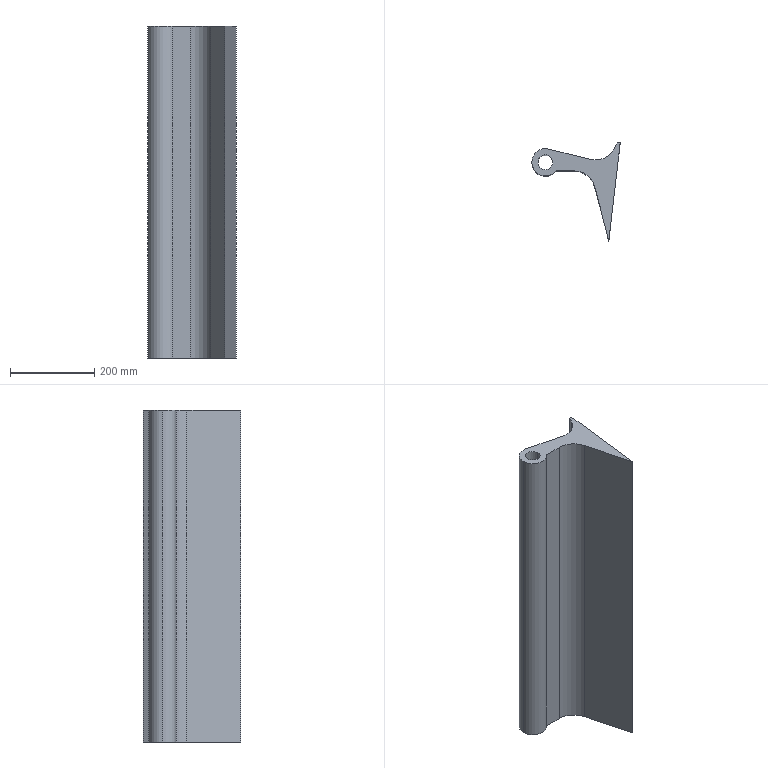Part | SolidWorks | features Fillet 2, Extrusion 1 | 1 solid | 14 faces | box 210.318 x 232.159 x 790 mm | volume 10438808 mm3 | plane 8 | cylinder 6 | commonest cylinder face diameters 35 x2 65 x2 100 x2
STEP:
#1=CARTESIAN_POINT('',(-17.5,0.,790.));
#2=VERTEX_POINT('',#1);
#3=CARTESIAN_POINT('',(17.5,0.,790.));
#4=VERTEX_POINT('',#3);
#5=CARTESIAN_POINT('',(0.,0.,790.));
#6=DIRECTION('',(0.,0.,1.));
#7=DIRECTION('',(1.,0.,0.));
#8=AXIS2_PLACEMENT_3D('',#5,#6,#7);
#9=CIRCLE('',#8,17.5);
#10=EDGE_CURVE('',#2,#4,#9,.T.);
#11=ORIENTED_EDGE('',*,*,#10,.T.);
#12=CARTESIAN_POINT('',(17.5,0.,0.));
#13=VERTEX_POINT('',#12);
#14=CARTESIAN_POINT('',(17.5,0.,790.));
#15=DIRECTION('',(0.,0.,-1.));
#16=VECTOR('',#15,1000.);
#17=LINE('',#14,#16);
#18=EDGE_CURVE('',#4,#13,#17,.T.);
#19=ORIENTED_EDGE('',*,*,#18,.T.);
#20=CARTESIAN_POINT('',(-17.5,0.,0.));
#21=VERTEX_POINT('',#20);
#22=CARTESIAN_POINT('',(0.,0.,0.));
#23=DIRECTION('',(0.,0.,1.));
#24=DIRECTION('',(1.,0.,0.));
#25=AXIS2_PLACEMENT_3D('',#22,#23,#24);
#26=CIRCLE('',#25,17.5);
#27=EDGE_CURVE('',#21,#13,#26,.T.);
#28=ORIENTED_EDGE('',*,*,#27,.F.);
#29=CARTESIAN_POINT('',(-17.5,0.,790.));
#30=DIRECTION('',(0.,0.,-1.));
#31=VECTOR('',#30,1000.);
#32=LINE('',#29,#31);
#33=EDGE_CURVE('',#2,#21,#32,.T.);
#34=ORIENTED_EDGE('',*,*,#33,.F.);
#35=EDGE_LOOP('',(#11,#19,#28,#34));
#36=FACE_OUTER_BOUND('',#35,.T.);
#37=CARTESIAN_POINT('',(0.,0.,790.));
#38=DIRECTION('',(0.,0.,-1.));
#39=DIRECTION('',(-1.,0.,0.));
#40=AXIS2_PLACEMENT_3D('',#37,#38,#39);
#41=CYLINDRICAL_SURFACE('',#40,17.5);
#42=ADVANCED_FACE('',(#36),#41,.F.);
#43=CARTESIAN_POINT('',(-32.5,0.,790.));
#44=VERTEX_POINT('',#43);
#45=CARTESIAN_POINT('',(25.188,-20.539,790.));
#46=VERTEX_POINT('',#45);
#47=CARTESIAN_POINT('',(0.,0.,790.));
#48=DIRECTION('',(0.,0.,1.));
#49=DIRECTION('',(1.,0.,0.));
#50=AXIS2_PLACEMENT_3D('',#47,#48,#49);
#51=CIRCLE('',#50,32.5);
#52=EDGE_CURVE('',#44,#46,#51,.T.);
#53=ORIENTED_EDGE('',*,*,#52,.F.);
#54=CARTESIAN_POINT('',(-32.5,0.,0.));
#55=VERTEX_POINT('',#54);
#56=CARTESIAN_POINT('',(-32.5,0.,790.));
#57=DIRECTION('',(0.,0.,-1.));
#58=VECTOR('',#57,1000.);
#59=LINE('',#56,#58);
#60=EDGE_CURVE('',#44,#55,#59,.T.);
#61=ORIENTED_EDGE('',*,*,#60,.T.);
#62=CARTESIAN_POINT('',(25.188,-20.539,0.));
#63=VERTEX_POINT('',#62);
#64=CARTESIAN_POINT('',(0.,0.,0.));
#65=DIRECTION('',(0.,0.,1.));
#66=DIRECTION('',(1.,0.,0.));
#67=AXIS2_PLACEMENT_3D('',#64,#65,#66);
#68=CIRCLE('',#67,32.5);
#69=EDGE_CURVE('',#55,#63,#68,.T.);
#70=ORIENTED_EDGE('',*,*,#69,.T.);
#71=CARTESIAN_POINT('',(25.188,-20.539,790.));
#72=DIRECTION('',(0.,0.,-1.));
#73=VECTOR('',#72,1000.);
#74=LINE('',#71,#73);
#75=EDGE_CURVE('',#46,#63,#74,.T.);
#76=ORIENTED_EDGE('',*,*,#75,.F.);
#77=EDGE_LOOP('',(#53,#61,#70,#76));
#78=FACE_OUTER_BOUND('',#77,.T.);
#79=CARTESIAN_POINT('',(0.,0.,790.));
#80=DIRECTION('',(0.,0.,-1.));
#81=DIRECTION('',(-1.,0.,0.));
#82=AXIS2_PLACEMENT_3D('',#79,#80,#81);
#83=CYLINDRICAL_SURFACE('',#82,32.5);
#84=ADVANCED_FACE('',(#78),#83,.T.);
#85=CARTESIAN_POINT('',(150.623,-186.13,790.));
#86=VERTEX_POINT('',#85);
#87=CARTESIAN_POINT('',(177.818,46.028,790.));
#88=VERTEX_POINT('',#87);
#89=CARTESIAN_POINT('',(150.623,-186.13,790.));
#90=DIRECTION('',(0.1163,0.9932,0.));
#91=VECTOR('',#90,1000.);
#92=LINE('',#89,#91);
#93=EDGE_CURVE('',#86,#88,#92,.T.);
#94=ORIENTED_EDGE('',*,*,#93,.T.);
#95=CARTESIAN_POINT('',(170.412,46.028,790.));
#96=VERTEX_POINT('',#95);
#97=CARTESIAN_POINT('',(177.818,46.028,790.));
#98=DIRECTION('',(-1.,0.,0.));
#99=VECTOR('',#98,1000.);
#100=LINE('',#97,#99);
#101=EDGE_CURVE('',#88,#96,#100,.T.);
#102=ORIENTED_EDGE('',*,*,#101,.T.);
#103=CARTESIAN_POINT('',(163.403,32.535,790.));
#104=VERTEX_POINT('',#103);
#105=CARTESIAN_POINT('',(145.258,-2.393,790.));
#106=DIRECTION('',(-0.461,-0.8874,0.));
#107=VECTOR('',#106,1000.);
#108=LINE('',#105,#107);
#109=EDGE_CURVE('',#96,#104,#108,.T.);
#110=ORIENTED_EDGE('',*,*,#109,.T.);
#111=CARTESIAN_POINT('',(107.046,7.043,790.));
#112=VERTEX_POINT('',#111);
#113=CARTESIAN_POINT('',(119.033,55.585,790.));
#114=DIRECTION('',(0.,0.,-1.));
#115=DIRECTION('',(1.,0.,0.));
#116=AXIS2_PLACEMENT_3D('',#113,#114,#115);
#117=CIRCLE('',#116,50.);
#118=EDGE_CURVE('',#104,#112,#117,.T.);
#119=ORIENTED_EDGE('',*,*,#118,.T.);
#120=CARTESIAN_POINT('',(7.791,31.552,790.));
#121=VERTEX_POINT('',#120);
#122=CARTESIAN_POINT('',(7.791,31.552,790.));
#123=DIRECTION('',(-0.9708,0.2397,0.));
#124=VECTOR('',#123,1000.);
#125=LINE('',#122,#124);
#126=EDGE_CURVE('',#112,#121,#125,.T.);
#127=ORIENTED_EDGE('',*,*,#126,.T.);
#128=CARTESIAN_POINT('',(0.,0.,790.));
#129=DIRECTION('',(0.,0.,1.));
#130=DIRECTION('',(1.,0.,0.));
#131=AXIS2_PLACEMENT_3D('',#128,#129,#130);
#132=CIRCLE('',#131,32.5);
#133=EDGE_CURVE('',#121,#44,#132,.T.);
#134=ORIENTED_EDGE('',*,*,#133,.T.);
#135=ORIENTED_EDGE('',*,*,#52,.T.);
#136=CARTESIAN_POINT('',(68.802,-20.539,790.));
#137=VERTEX_POINT('',#136);
#138=CARTESIAN_POINT('',(107.434,-20.539,790.));
#139=DIRECTION('',(1.,0.,0.));
#140=VECTOR('',#139,1000.);
#141=LINE('',#138,#140);
#142=EDGE_CURVE('',#46,#137,#141,.T.);
#143=ORIENTED_EDGE('',*,*,#142,.T.);
#144=CARTESIAN_POINT('',(117.184,-57.92,790.));
#145=VERTEX_POINT('',#144);
#146=CARTESIAN_POINT('',(68.802,-70.539,790.));
#147=DIRECTION('',(0.,0.,-1.));
#148=DIRECTION('',(1.,0.,0.));
#149=AXIS2_PLACEMENT_3D('',#146,#147,#148);
#150=CIRCLE('',#149,50.);
#151=EDGE_CURVE('',#137,#145,#150,.T.);
#152=ORIENTED_EDGE('',*,*,#151,.T.);
#153=CARTESIAN_POINT('',(107.434,-20.539,790.));
#154=DIRECTION('',(0.2524,-0.9676,0.));
#155=VECTOR('',#154,1000.);
#156=LINE('',#153,#155);
#157=EDGE_CURVE('',#145,#86,#156,.T.);
#158=ORIENTED_EDGE('',*,*,#157,.T.);
#159=EDGE_LOOP('',(#94,#102,#110,#119,#127,#134,#135,#143,#152,#158));
#160=FACE_OUTER_BOUND('',#159,.T.);
#161=ORIENTED_EDGE('',*,*,#10,.F.);
#162=CARTESIAN_POINT('',(0.,0.,790.));
#163=DIRECTION('',(0.,0.,1.));
#164=DIRECTION('',(1.,0.,0.));
#165=AXIS2_PLACEMENT_3D('',#162,#163,#164);
#166=CIRCLE('',#165,17.5);
#167=EDGE_CURVE('',#4,#2,#166,.T.);
#168=ORIENTED_EDGE('',*,*,#167,.F.);
#169=EDGE_LOOP('',(#161,#168));
#170=FACE_BOUND('',#169,.T.);
#171=CARTESIAN_POINT('',(0.,0.,790.));
#172=DIRECTION('',(0.,0.,1.));
#173=DIRECTION('',(1.,0.,0.));
#174=AXIS2_PLACEMENT_3D('',#171,#172,#173);
#175=PLANE('',#174);
#176=ADVANCED_FACE('',(#160,#170),#175,.T.);
#177=CARTESIAN_POINT('',(150.623,-186.13,0.));
#178=VERTEX_POINT('',#177);
#179=CARTESIAN_POINT('',(177.818,46.028,0.));
#180=VERTEX_POINT('',#179);
#181=CARTESIAN_POINT('',(150.623,-186.13,0.));
#182=DIRECTION('',(0.1163,0.9932,0.));
#183=VECTOR('',#182,1000.);
#184=LINE('',#181,#183);
#185=EDGE_CURVE('',#178,#180,#184,.T.);
#186=ORIENTED_EDGE('',*,*,#185,.F.);
#187=CARTESIAN_POINT('',(117.184,-57.92,0.));
#188=VERTEX_POINT('',#187);
#189=CARTESIAN_POINT('',(107.434,-20.539,0.));
#190=DIRECTION('',(0.2524,-0.9676,0.));
#191=VECTOR('',#190,1000.);
#192=LINE('',#189,#191);
#193=EDGE_CURVE('',#188,#178,#192,.T.);
#194=ORIENTED_EDGE('',*,*,#193,.F.);
#195=CARTESIAN_POINT('',(68.802,-20.539,0.));
#196=VERTEX_POINT('',#195);
#197=CARTESIAN_POINT('',(68.802,-70.539,0.));
#198=DIRECTION('',(0.,0.,1.));
#199=DIRECTION('',(1.,0.,0.));
#200=AXIS2_PLACEMENT_3D('',#197,#198,#199);
#201=CIRCLE('',#200,50.);
#202=EDGE_CURVE('',#188,#196,#201,.T.);
#203=ORIENTED_EDGE('',*,*,#202,.T.);
#204=CARTESIAN_POINT('',(107.434,-20.539,0.));
#205=DIRECTION('',(1.,0.,0.));
#206=VECTOR('',#205,1000.);
#207=LINE('',#204,#206);
#208=EDGE_CURVE('',#63,#196,#207,.T.);
#209=ORIENTED_EDGE('',*,*,#208,.F.);
#210=ORIENTED_EDGE('',*,*,#69,.F.);
#211=CARTESIAN_POINT('',(7.791,31.552,0.));
#212=VERTEX_POINT('',#211);
#213=CARTESIAN_POINT('',(0.,0.,0.));
#214=DIRECTION('',(0.,0.,1.));
#215=DIRECTION('',(1.,0.,0.));
#216=AXIS2_PLACEMENT_3D('',#213,#214,#215);
#217=CIRCLE('',#216,32.5);
#218=EDGE_CURVE('',#212,#55,#217,.T.);
#219=ORIENTED_EDGE('',*,*,#218,.F.);
#220=CARTESIAN_POINT('',(107.046,7.043,0.));
#221=VERTEX_POINT('',#220);
#222=CARTESIAN_POINT('',(7.791,31.552,0.));
#223=DIRECTION('',(-0.9708,0.2397,0.));
#224=VECTOR('',#223,1000.);
#225=LINE('',#222,#224);
#226=EDGE_CURVE('',#221,#212,#225,.T.);
#227=ORIENTED_EDGE('',*,*,#226,.F.);
#228=CARTESIAN_POINT('',(163.403,32.535,0.));
#229=VERTEX_POINT('',#228);
#230=CARTESIAN_POINT('',(119.033,55.585,0.));
#231=DIRECTION('',(0.,0.,1.));
#232=DIRECTION('',(1.,0.,0.));
#233=AXIS2_PLACEMENT_3D('',#230,#231,#232);
#234=CIRCLE('',#233,50.);
#235=EDGE_CURVE('',#221,#229,#234,.T.);
#236=ORIENTED_EDGE('',*,*,#235,.T.);
#237=CARTESIAN_POINT('',(170.412,46.028,0.));
#238=VERTEX_POINT('',#237);
#239=CARTESIAN_POINT('',(145.258,-2.393,0.));
#240=DIRECTION('',(-0.461,-0.8874,0.));
#241=VECTOR('',#240,1000.);
#242=LINE('',#239,#241);
#243=EDGE_CURVE('',#238,#229,#242,.T.);
#244=ORIENTED_EDGE('',*,*,#243,.F.);
#245=CARTESIAN_POINT('',(177.818,46.028,0.));
#246=DIRECTION('',(-1.,0.,0.));
#247=VECTOR('',#246,1000.);
#248=LINE('',#245,#247);
#249=EDGE_CURVE('',#180,#238,#248,.T.);
#250=ORIENTED_EDGE('',*,*,#249,.F.);
#251=EDGE_LOOP('',(#186,#194,#203,#209,#210,#219,#227,#236,#244,#250));
#252=FACE_OUTER_BOUND('',#251,.T.);
#253=ORIENTED_EDGE('',*,*,#27,.T.);
#254=CARTESIAN_POINT('',(0.,0.,0.));
#255=DIRECTION('',(0.,0.,1.));
#256=DIRECTION('',(1.,0.,0.));
#257=AXIS2_PLACEMENT_3D('',#254,#255,#256);
#258=CIRCLE('',#257,17.5);
#259=EDGE_CURVE('',#13,#21,#258,.T.);
#260=ORIENTED_EDGE('',*,*,#259,.T.);
#261=EDGE_LOOP('',(#253,#260));
#262=FACE_BOUND('',#261,.T.);
#263=CARTESIAN_POINT('',(0.,0.,0.));
#264=DIRECTION('',(0.,0.,1.));
#265=DIRECTION('',(1.,0.,0.));
#266=AXIS2_PLACEMENT_3D('',#263,#264,#265);
#267=PLANE('',#266);
#268=ADVANCED_FACE('',(#252,#262),#267,.F.);
#269=ORIENTED_EDGE('',*,*,#185,.T.);
#270=CARTESIAN_POINT('',(177.818,46.028,790.));
#271=DIRECTION('',(0.,0.,-1.));
#272=VECTOR('',#271,1000.);
#273=LINE('',#270,#272);
#274=EDGE_CURVE('',#88,#180,#273,.T.);
#275=ORIENTED_EDGE('',*,*,#274,.F.);
#276=ORIENTED_EDGE('',*,*,#93,.F.);
#277=CARTESIAN_POINT('',(150.623,-186.13,790.));
#278=DIRECTION('',(0.,0.,-1.));
#279=VECTOR('',#278,1000.);
#280=LINE('',#277,#279);
#281=EDGE_CURVE('',#86,#178,#280,.T.);
#282=ORIENTED_EDGE('',*,*,#281,.T.);
#283=EDGE_LOOP('',(#269,#275,#276,#282));
#284=FACE_OUTER_BOUND('',#283,.T.);
#285=CARTESIAN_POINT('',(150.623,-186.13,790.));
#286=DIRECTION('',(-0.9932,0.1163,0.));
#287=DIRECTION('',(-0.1163,-0.9932,0.));
#288=AXIS2_PLACEMENT_3D('',#285,#286,#287);
#289=PLANE('',#288);
#290=ADVANCED_FACE('',(#284),#289,.F.);
#291=ORIENTED_EDGE('',*,*,#249,.T.);
#292=CARTESIAN_POINT('',(170.412,46.028,790.));
#293=DIRECTION('',(0.,0.,-1.));
#294=VECTOR('',#293,1000.);
#295=LINE('',#292,#294);
#296=EDGE_CURVE('',#96,#238,#295,.T.);
#297=ORIENTED_EDGE('',*,*,#296,.F.);
#298=ORIENTED_EDGE('',*,*,#101,.F.);
#299=ORIENTED_EDGE('',*,*,#274,.T.);
#300=EDGE_LOOP('',(#291,#297,#298,#299));
#301=FACE_OUTER_BOUND('',#300,.T.);
#302=CARTESIAN_POINT('',(177.818,46.028,790.));
#303=DIRECTION('',(0.,-1.,0.));
#304=DIRECTION('',(0.,0.,-1.));
#305=AXIS2_PLACEMENT_3D('',#302,#303,#304);
#306=PLANE('',#305);
#307=ADVANCED_FACE('',(#301),#306,.F.);
#308=ORIENTED_EDGE('',*,*,#243,.T.);
#309=CARTESIAN_POINT('',(163.403,32.535,790.));
#310=DIRECTION('',(0.,0.,1.));
#311=VECTOR('',#310,1000.);
#312=LINE('',#309,#311);
#313=EDGE_CURVE('',#229,#104,#312,.T.);
#314=ORIENTED_EDGE('',*,*,#313,.T.);
#315=ORIENTED_EDGE('',*,*,#109,.F.);
#316=ORIENTED_EDGE('',*,*,#296,.T.);
#317=EDGE_LOOP('',(#308,#314,#315,#316));
#318=FACE_OUTER_BOUND('',#317,.T.);
#319=CARTESIAN_POINT('',(145.258,-2.393,790.));
#320=DIRECTION('',(0.8874,-0.461,0.));
#321=DIRECTION('',(0.461,0.8874,0.));
#322=AXIS2_PLACEMENT_3D('',#319,#320,#321);
#323=PLANE('',#322);
#324=ADVANCED_FACE('',(#318),#323,.F.);
#325=ORIENTED_EDGE('',*,*,#126,.F.);
#326=CARTESIAN_POINT('',(107.046,7.043,0.));
#327=DIRECTION('',(0.,0.,-1.));
#328=VECTOR('',#327,1000.);
#329=LINE('',#326,#328);
#330=EDGE_CURVE('',#112,#221,#329,.T.);
#331=ORIENTED_EDGE('',*,*,#330,.T.);
#332=ORIENTED_EDGE('',*,*,#226,.T.);
#333=CARTESIAN_POINT('',(7.791,31.552,790.));
#334=DIRECTION('',(0.,0.,-1.));
#335=VECTOR('',#334,1000.);
#336=LINE('',#333,#335);
#337=EDGE_CURVE('',#121,#212,#336,.T.);
#338=ORIENTED_EDGE('',*,*,#337,.F.);
#339=EDGE_LOOP('',(#325,#331,#332,#338));
#340=FACE_OUTER_BOUND('',#339,.T.);
#341=CARTESIAN_POINT('',(7.791,31.552,790.));
#342=DIRECTION('',(-0.2397,-0.9708,0.));
#343=DIRECTION('',(0.9708,-0.2397,0.));
#344=AXIS2_PLACEMENT_3D('',#341,#342,#343);
#345=PLANE('',#344);
#346=ADVANCED_FACE('',(#340),#345,.F.);
#347=ORIENTED_EDGE('',*,*,#60,.F.);
#348=ORIENTED_EDGE('',*,*,#133,.F.);
#349=ORIENTED_EDGE('',*,*,#337,.T.);
#350=ORIENTED_EDGE('',*,*,#218,.T.);
#351=EDGE_LOOP('',(#347,#348,#349,#350));
#352=FACE_OUTER_BOUND('',#351,.T.);
#353=CARTESIAN_POINT('',(0.,0.,790.));
#354=DIRECTION('',(0.,0.,-1.));
#355=DIRECTION('',(-1.,0.,0.));
#356=AXIS2_PLACEMENT_3D('',#353,#354,#355);
#357=CYLINDRICAL_SURFACE('',#356,32.5);
#358=ADVANCED_FACE('',(#352),#357,.T.);
#359=ORIENTED_EDGE('',*,*,#208,.T.);
#360=CARTESIAN_POINT('',(68.802,-20.539,790.));
#361=DIRECTION('',(0.,0.,1.));
#362=VECTOR('',#361,1000.);
#363=LINE('',#360,#362);
#364=EDGE_CURVE('',#196,#137,#363,.T.);
#365=ORIENTED_EDGE('',*,*,#364,.T.);
#366=ORIENTED_EDGE('',*,*,#142,.F.);
#367=ORIENTED_EDGE('',*,*,#75,.T.);
#368=EDGE_LOOP('',(#359,#365,#366,#367));
#369=FACE_OUTER_BOUND('',#368,.T.);
#370=CARTESIAN_POINT('',(107.434,-20.539,790.));
#371=DIRECTION('',(0.,1.,0.));
#372=DIRECTION('',(-1.,0.,0.));
#373=AXIS2_PLACEMENT_3D('',#370,#371,#372);
#374=PLANE('',#373);
#375=ADVANCED_FACE('',(#369),#374,.F.);
#376=ORIENTED_EDGE('',*,*,#157,.F.);
#377=CARTESIAN_POINT('',(117.184,-57.92,0.));
#378=DIRECTION('',(0.,0.,-1.));
#379=VECTOR('',#378,1000.);
#380=LINE('',#377,#379);
#381=EDGE_CURVE('',#145,#188,#380,.T.);
#382=ORIENTED_EDGE('',*,*,#381,.T.);
#383=ORIENTED_EDGE('',*,*,#193,.T.);
#384=ORIENTED_EDGE('',*,*,#281,.F.);
#385=EDGE_LOOP('',(#376,#382,#383,#384));
#386=FACE_OUTER_BOUND('',#385,.T.);
#387=CARTESIAN_POINT('',(107.434,-20.539,790.));
#388=DIRECTION('',(0.9676,0.2524,0.));
#389=DIRECTION('',(-0.2524,0.9676,0.));
#390=AXIS2_PLACEMENT_3D('',#387,#388,#389);
#391=PLANE('',#390);
#392=ADVANCED_FACE('',(#386),#391,.F.);
#393=ORIENTED_EDGE('',*,*,#18,.F.);
#394=ORIENTED_EDGE('',*,*,#167,.T.);
#395=ORIENTED_EDGE('',*,*,#33,.T.);
#396=ORIENTED_EDGE('',*,*,#259,.F.);
#397=EDGE_LOOP('',(#393,#394,#395,#396));
#398=FACE_OUTER_BOUND('',#397,.T.);
#399=CARTESIAN_POINT('',(0.,0.,790.));
#400=DIRECTION('',(0.,0.,-1.));
#401=DIRECTION('',(-1.,0.,0.));
#402=AXIS2_PLACEMENT_3D('',#399,#400,#401);
#403=CYLINDRICAL_SURFACE('',#402,17.5);
#404=ADVANCED_FACE('',(#398),#403,.F.);
#405=ORIENTED_EDGE('',*,*,#118,.F.);
#406=ORIENTED_EDGE('',*,*,#313,.F.);
#407=ORIENTED_EDGE('',*,*,#235,.F.);
#408=ORIENTED_EDGE('',*,*,#330,.F.);
#409=EDGE_LOOP('',(#405,#406,#407,#408));
#410=FACE_OUTER_BOUND('',#409,.T.);
#411=CARTESIAN_POINT('',(119.033,55.585,790.));
#412=DIRECTION('',(0.,0.,1.));
#413=DIRECTION('',(1.,0.,0.));
#414=AXIS2_PLACEMENT_3D('',#411,#412,#413);
#415=CYLINDRICAL_SURFACE('',#414,50.);
#416=ADVANCED_FACE('',(#410),#415,.F.);
#417=ORIENTED_EDGE('',*,*,#151,.F.);
#418=ORIENTED_EDGE('',*,*,#364,.F.);
#419=ORIENTED_EDGE('',*,*,#202,.F.);
#420=ORIENTED_EDGE('',*,*,#381,.F.);
#421=EDGE_LOOP('',(#417,#418,#419,#420));
#422=FACE_OUTER_BOUND('',#421,.T.);
#423=CARTESIAN_POINT('',(68.802,-70.539,790.));
#424=DIRECTION('',(0.,0.,1.));
#425=DIRECTION('',(1.,0.,0.));
#426=AXIS2_PLACEMENT_3D('',#423,#424,#425);
#427=CYLINDRICAL_SURFACE('',#426,50.);
#428=ADVANCED_FACE('',(#422),#427,.F.);
#429=CLOSED_SHELL('',(#42,#84,#176,#268,#290,#307,#324,#346,#358,#375,#392,#404,#416,#428));
#430=MANIFOLD_SOLID_BREP('',#429);
#431=CARTESIAN_POINT('',(0.,0.,0.));
#432=DIRECTION('',(0.,0.,1.));
#433=DIRECTION('',(1.,0.,0.));
#434=AXIS2_PLACEMENT_3D('',#431,#432,#433);
#435=(LENGTH_UNIT()NAMED_UNIT(*)SI_UNIT(.MILLI.,.METRE.));
#436=UNCERTAINTY_MEASURE_WITH_UNIT(LENGTH_MEASURE(0.00001),#435,'','');
#437=(NAMED_UNIT(*)PLANE_ANGLE_UNIT()SI_UNIT($,.RADIAN.));
#438=(NAMED_UNIT(*)SI_UNIT($,.STERADIAN.)SOLID_ANGLE_UNIT());
#439=(GEOMETRIC_REPRESENTATION_CONTEXT(3)GLOBAL_UNCERTAINTY_ASSIGNED_CONTEXT((#436))GLOBAL_UNIT_ASSIGNED_CONTEXT((#435,#437,#438))REPRESENTATION_CONTEXT('',''));
#440=ADVANCED_BREP_SHAPE_REPRESENTATION('',(#430,#434),#439);